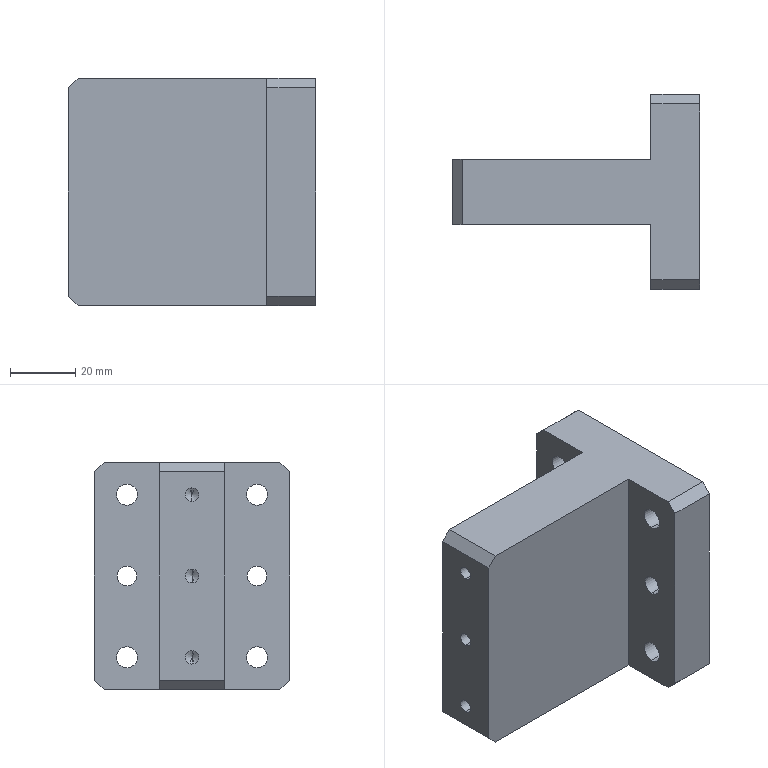Part | STEP file | 10-23 sliding mounting seat | 1 solid | 40 faces | box 76 x 60 x 70 mm | volume 144578 mm3 | cylinder 18 | plane 16 | cone 6 | commonest cylinder face diameters 6.5 x8 4.2 x6 6 x4
STEP:
#1=CARTESIAN_POINT('',(-48.6,0.,-27.1));
#2=VERTEX_POINT('',#1);
#3=CARTESIAN_POINT('',(-48.6,0.,-22.9));
#4=VERTEX_POINT('',#3);
#5=CARTESIAN_POINT('',(-48.6,0.,-25.));
#6=DIRECTION('',(-1.,0.,0.));
#7=DIRECTION('',(0.,0.,1.));
#8=AXIS2_PLACEMENT_3D('',#5,#6,#7);
#9=CIRCLE('',#8,2.1);
#10=EDGE_CURVE('',#2,#4,#9,.T.);
#11=ORIENTED_EDGE('',*,*,#10,.F.);
#12=CARTESIAN_POINT('',(-61.,0.,-27.1));
#13=VERTEX_POINT('',#12);
#14=CARTESIAN_POINT('',(-61.,0.,-27.1));
#15=DIRECTION('',(-1.,0.,0.));
#16=VECTOR('',#15,1000.);
#17=LINE('',#14,#16);
#18=EDGE_CURVE('',#2,#13,#17,.T.);
#19=ORIENTED_EDGE('',*,*,#18,.T.);
#20=CARTESIAN_POINT('',(-61.,0.,-22.9));
#21=VERTEX_POINT('',#20);
#22=CARTESIAN_POINT('',(-61.,0.,-25.));
#23=DIRECTION('',(-1.,0.,0.));
#24=DIRECTION('',(0.,0.,1.));
#25=AXIS2_PLACEMENT_3D('',#22,#23,#24);
#26=CIRCLE('',#25,2.1);
#27=EDGE_CURVE('',#13,#21,#26,.T.);
#28=ORIENTED_EDGE('',*,*,#27,.T.);
#29=CARTESIAN_POINT('',(-61.,0.,-22.9));
#30=DIRECTION('',(-1.,0.,0.));
#31=VECTOR('',#30,1000.);
#32=LINE('',#29,#31);
#33=EDGE_CURVE('',#4,#21,#32,.T.);
#34=ORIENTED_EDGE('',*,*,#33,.F.);
#35=EDGE_LOOP('',(#11,#19,#28,#34));
#36=FACE_OUTER_BOUND('',#35,.T.);
#37=CARTESIAN_POINT('',(-61.,0.,-25.));
#38=DIRECTION('',(-1.,0.,0.));
#39=DIRECTION('',(0.,0.,1.));
#40=AXIS2_PLACEMENT_3D('',#37,#38,#39);
#41=CYLINDRICAL_SURFACE('',#40,2.1);
#42=ADVANCED_FACE('',(#36),#41,.F.);
#43=CARTESIAN_POINT('',(-47.338,0.,-25.));
#44=VERTEX_POINT('',#43);
#45=CARTESIAN_POINT('',(-48.6,0.,-22.9));
#46=DIRECTION('',(-0.515,0.,0.8572));
#47=VECTOR('',#46,1000.);
#48=LINE('',#45,#47);
#49=EDGE_CURVE('',#44,#4,#48,.T.);
#50=ORIENTED_EDGE('',*,*,#49,.F.);
#51=CARTESIAN_POINT('',(-48.6,0.,-27.1));
#52=DIRECTION('',(-0.515,0.,-0.8572));
#53=VECTOR('',#52,1000.);
#54=LINE('',#51,#53);
#55=EDGE_CURVE('',#44,#2,#54,.T.);
#56=ORIENTED_EDGE('',*,*,#55,.T.);
#57=ORIENTED_EDGE('',*,*,#10,.T.);
#58=EDGE_LOOP('',(#50,#56,#57));
#59=FACE_OUTER_BOUND('',#58,.T.);
#60=CARTESIAN_POINT('',(-48.6,0.,-25.));
#61=DIRECTION('',(-1.,0.,0.));
#62=DIRECTION('',(0.,0.,1.));
#63=AXIS2_PLACEMENT_3D('',#60,#61,#62);
#64=CONICAL_SURFACE('',#63,2.1,1.03);
#65=ADVANCED_FACE('',(#59),#64,.F.);
#66=CARTESIAN_POINT('',(-48.6,0.,-2.1));
#67=VERTEX_POINT('',#66);
#68=CARTESIAN_POINT('',(-48.6,0.,2.1));
#69=VERTEX_POINT('',#68);
#70=CARTESIAN_POINT('',(-48.6,0.,0.));
#71=DIRECTION('',(-1.,0.,0.));
#72=DIRECTION('',(0.,0.,1.));
#73=AXIS2_PLACEMENT_3D('',#70,#71,#72);
#74=CIRCLE('',#73,2.1);
#75=EDGE_CURVE('',#67,#69,#74,.T.);
#76=ORIENTED_EDGE('',*,*,#75,.F.);
#77=CARTESIAN_POINT('',(-61.,0.,-2.1));
#78=VERTEX_POINT('',#77);
#79=CARTESIAN_POINT('',(-61.,0.,-2.1));
#80=DIRECTION('',(-1.,0.,0.));
#81=VECTOR('',#80,1000.);
#82=LINE('',#79,#81);
#83=EDGE_CURVE('',#67,#78,#82,.T.);
#84=ORIENTED_EDGE('',*,*,#83,.T.);
#85=CARTESIAN_POINT('',(-61.,0.,2.1));
#86=VERTEX_POINT('',#85);
#87=CARTESIAN_POINT('',(-61.,0.,0.));
#88=DIRECTION('',(-1.,0.,0.));
#89=DIRECTION('',(0.,0.,1.));
#90=AXIS2_PLACEMENT_3D('',#87,#88,#89);
#91=CIRCLE('',#90,2.1);
#92=EDGE_CURVE('',#78,#86,#91,.T.);
#93=ORIENTED_EDGE('',*,*,#92,.T.);
#94=CARTESIAN_POINT('',(-61.,0.,2.1));
#95=DIRECTION('',(-1.,0.,0.));
#96=VECTOR('',#95,1000.);
#97=LINE('',#94,#96);
#98=EDGE_CURVE('',#69,#86,#97,.T.);
#99=ORIENTED_EDGE('',*,*,#98,.F.);
#100=EDGE_LOOP('',(#76,#84,#93,#99));
#101=FACE_OUTER_BOUND('',#100,.T.);
#102=CARTESIAN_POINT('',(-61.,0.,0.));
#103=DIRECTION('',(-1.,0.,0.));
#104=DIRECTION('',(0.,0.,1.));
#105=AXIS2_PLACEMENT_3D('',#102,#103,#104);
#106=CYLINDRICAL_SURFACE('',#105,2.1);
#107=ADVANCED_FACE('',(#101),#106,.F.);
#108=CARTESIAN_POINT('',(-47.338,0.,0.));
#109=VERTEX_POINT('',#108);
#110=CARTESIAN_POINT('',(-48.6,0.,2.1));
#111=DIRECTION('',(-0.515,0.,0.8572));
#112=VECTOR('',#111,1000.);
#113=LINE('',#110,#112);
#114=EDGE_CURVE('',#109,#69,#113,.T.);
#115=ORIENTED_EDGE('',*,*,#114,.F.);
#116=CARTESIAN_POINT('',(-48.6,0.,-2.1));
#117=DIRECTION('',(-0.515,0.,-0.8572));
#118=VECTOR('',#117,1000.);
#119=LINE('',#116,#118);
#120=EDGE_CURVE('',#109,#67,#119,.T.);
#121=ORIENTED_EDGE('',*,*,#120,.T.);
#122=ORIENTED_EDGE('',*,*,#75,.T.);
#123=EDGE_LOOP('',(#115,#121,#122));
#124=FACE_OUTER_BOUND('',#123,.T.);
#125=CARTESIAN_POINT('',(-48.6,0.,0.));
#126=DIRECTION('',(-1.,0.,0.));
#127=DIRECTION('',(0.,0.,1.));
#128=AXIS2_PLACEMENT_3D('',#125,#126,#127);
#129=CONICAL_SURFACE('',#128,2.1,1.03);
#130=ADVANCED_FACE('',(#124),#129,.F.);
#131=CARTESIAN_POINT('',(-48.6,0.,22.9));
#132=VERTEX_POINT('',#131);
#133=CARTESIAN_POINT('',(-48.6,0.,27.1));
#134=VERTEX_POINT('',#133);
#135=CARTESIAN_POINT('',(-48.6,0.,25.));
#136=DIRECTION('',(-1.,0.,0.));
#137=DIRECTION('',(0.,0.,1.));
#138=AXIS2_PLACEMENT_3D('',#135,#136,#137);
#139=CIRCLE('',#138,2.1);
#140=EDGE_CURVE('',#132,#134,#139,.T.);
#141=ORIENTED_EDGE('',*,*,#140,.F.);
#142=CARTESIAN_POINT('',(-61.,0.,22.9));
#143=VERTEX_POINT('',#142);
#144=CARTESIAN_POINT('',(-61.,0.,22.9));
#145=DIRECTION('',(-1.,0.,0.));
#146=VECTOR('',#145,1000.);
#147=LINE('',#144,#146);
#148=EDGE_CURVE('',#132,#143,#147,.T.);
#149=ORIENTED_EDGE('',*,*,#148,.T.);
#150=CARTESIAN_POINT('',(-61.,0.,27.1));
#151=VERTEX_POINT('',#150);
#152=CARTESIAN_POINT('',(-61.,0.,25.));
#153=DIRECTION('',(-1.,0.,0.));
#154=DIRECTION('',(0.,0.,1.));
#155=AXIS2_PLACEMENT_3D('',#152,#153,#154);
#156=CIRCLE('',#155,2.1);
#157=EDGE_CURVE('',#143,#151,#156,.T.);
#158=ORIENTED_EDGE('',*,*,#157,.T.);
#159=CARTESIAN_POINT('',(-61.,0.,27.1));
#160=DIRECTION('',(-1.,0.,0.));
#161=VECTOR('',#160,1000.);
#162=LINE('',#159,#161);
#163=EDGE_CURVE('',#134,#151,#162,.T.);
#164=ORIENTED_EDGE('',*,*,#163,.F.);
#165=EDGE_LOOP('',(#141,#149,#158,#164));
#166=FACE_OUTER_BOUND('',#165,.T.);
#167=CARTESIAN_POINT('',(-61.,0.,25.));
#168=DIRECTION('',(-1.,0.,0.));
#169=DIRECTION('',(0.,0.,1.));
#170=AXIS2_PLACEMENT_3D('',#167,#168,#169);
#171=CYLINDRICAL_SURFACE('',#170,2.1);
#172=ADVANCED_FACE('',(#166),#171,.F.);
#173=CARTESIAN_POINT('',(-47.338,0.,25.));
#174=VERTEX_POINT('',#173);
#175=CARTESIAN_POINT('',(-48.6,0.,27.1));
#176=DIRECTION('',(-0.515,0.,0.8572));
#177=VECTOR('',#176,1000.);
#178=LINE('',#175,#177);
#179=EDGE_CURVE('',#174,#134,#178,.T.);
#180=ORIENTED_EDGE('',*,*,#179,.F.);
#181=CARTESIAN_POINT('',(-48.6,0.,22.9));
#182=DIRECTION('',(-0.515,0.,-0.8572));
#183=VECTOR('',#182,1000.);
#184=LINE('',#181,#183);
#185=EDGE_CURVE('',#174,#132,#184,.T.);
#186=ORIENTED_EDGE('',*,*,#185,.T.);
#187=ORIENTED_EDGE('',*,*,#140,.T.);
#188=EDGE_LOOP('',(#180,#186,#187));
#189=FACE_OUTER_BOUND('',#188,.T.);
#190=CARTESIAN_POINT('',(-48.6,0.,25.));
#191=DIRECTION('',(-1.,0.,0.));
#192=DIRECTION('',(0.,0.,1.));
#193=AXIS2_PLACEMENT_3D('',#190,#191,#192);
#194=CONICAL_SURFACE('',#193,2.1,1.03);
#195=ADVANCED_FACE('',(#189),#194,.F.);
#196=CARTESIAN_POINT('',(15.,20.,-3.));
#197=VERTEX_POINT('',#196);
#198=CARTESIAN_POINT('',(15.,20.,3.));
#199=VERTEX_POINT('',#198);
#200=CARTESIAN_POINT('',(15.,20.,0.));
#201=DIRECTION('',(-1.,0.,0.));
#202=DIRECTION('',(0.,0.,1.));
#203=AXIS2_PLACEMENT_3D('',#200,#201,#202);
#204=CIRCLE('',#203,3.);
#205=EDGE_CURVE('',#197,#199,#204,.T.);
#206=ORIENTED_EDGE('',*,*,#205,.F.);
#207=CARTESIAN_POINT('',(0.,20.,-3.));
#208=VERTEX_POINT('',#207);
#209=CARTESIAN_POINT('',(0.,20.,-3.));
#210=DIRECTION('',(-1.,0.,0.));
#211=VECTOR('',#210,1000.);
#212=LINE('',#209,#211);
#213=EDGE_CURVE('',#197,#208,#212,.T.);
#214=ORIENTED_EDGE('',*,*,#213,.T.);
#215=CARTESIAN_POINT('',(0.,20.,3.));
#216=VERTEX_POINT('',#215);
#217=CARTESIAN_POINT('',(0.,20.,0.));
#218=DIRECTION('',(-1.,0.,0.));
#219=DIRECTION('',(0.,0.,1.));
#220=AXIS2_PLACEMENT_3D('',#217,#218,#219);
#221=CIRCLE('',#220,3.);
#222=EDGE_CURVE('',#208,#216,#221,.T.);
#223=ORIENTED_EDGE('',*,*,#222,.T.);
#224=CARTESIAN_POINT('',(0.,20.,3.));
#225=DIRECTION('',(-1.,0.,0.));
#226=VECTOR('',#225,1000.);
#227=LINE('',#224,#226);
#228=EDGE_CURVE('',#199,#216,#227,.T.);
#229=ORIENTED_EDGE('',*,*,#228,.F.);
#230=EDGE_LOOP('',(#206,#214,#223,#229));
#231=FACE_OUTER_BOUND('',#230,.T.);
#232=CARTESIAN_POINT('',(0.,20.,0.));
#233=DIRECTION('',(-1.,0.,0.));
#234=DIRECTION('',(0.,0.,1.));
#235=AXIS2_PLACEMENT_3D('',#232,#233,#234);
#236=CYLINDRICAL_SURFACE('',#235,3.);
#237=ADVANCED_FACE('',(#231),#236,.F.);
#238=CARTESIAN_POINT('',(15.,-20.,-3.));
#239=VERTEX_POINT('',#238);
#240=CARTESIAN_POINT('',(15.,-20.,3.));
#241=VERTEX_POINT('',#240);
#242=CARTESIAN_POINT('',(15.,-20.,0.));
#243=DIRECTION('',(-1.,0.,0.));
#244=DIRECTION('',(0.,0.,1.));
#245=AXIS2_PLACEMENT_3D('',#242,#243,#244);
#246=CIRCLE('',#245,3.);
#247=EDGE_CURVE('',#239,#241,#246,.T.);
#248=ORIENTED_EDGE('',*,*,#247,.F.);
#249=CARTESIAN_POINT('',(0.,-20.,-3.));
#250=VERTEX_POINT('',#249);
#251=CARTESIAN_POINT('',(0.,-20.,-3.));
#252=DIRECTION('',(-1.,0.,0.));
#253=VECTOR('',#252,1000.);
#254=LINE('',#251,#253);
#255=EDGE_CURVE('',#239,#250,#254,.T.);
#256=ORIENTED_EDGE('',*,*,#255,.T.);
#257=CARTESIAN_POINT('',(0.,-20.,3.));
#258=VERTEX_POINT('',#257);
#259=CARTESIAN_POINT('',(0.,-20.,0.));
#260=DIRECTION('',(-1.,0.,0.));
#261=DIRECTION('',(0.,0.,1.));
#262=AXIS2_PLACEMENT_3D('',#259,#260,#261);
#263=CIRCLE('',#262,3.);
#264=EDGE_CURVE('',#250,#258,#263,.T.);
#265=ORIENTED_EDGE('',*,*,#264,.T.);
#266=CARTESIAN_POINT('',(0.,-20.,3.));
#267=DIRECTION('',(-1.,0.,0.));
#268=VECTOR('',#267,1000.);
#269=LINE('',#266,#268);
#270=EDGE_CURVE('',#241,#258,#269,.T.);
#271=ORIENTED_EDGE('',*,*,#270,.F.);
#272=EDGE_LOOP('',(#248,#256,#265,#271));
#273=FACE_OUTER_BOUND('',#272,.T.);
#274=CARTESIAN_POINT('',(0.,-20.,0.));
#275=DIRECTION('',(-1.,0.,0.));
#276=DIRECTION('',(0.,0.,1.));
#277=AXIS2_PLACEMENT_3D('',#274,#275,#276);
#278=CYLINDRICAL_SURFACE('',#277,3.);
#279=ADVANCED_FACE('',(#273),#278,.F.);
#280=CARTESIAN_POINT('',(15.,20.,-28.25));
#281=VERTEX_POINT('',#280);
#282=CARTESIAN_POINT('',(15.,20.,-21.75));
#283=VERTEX_POINT('',#282);
#284=CARTESIAN_POINT('',(15.,20.,-25.));
#285=DIRECTION('',(-1.,0.,0.));
#286=DIRECTION('',(0.,0.,1.));
#287=AXIS2_PLACEMENT_3D('',#284,#285,#286);
#288=CIRCLE('',#287,3.25);
#289=EDGE_CURVE('',#281,#283,#288,.T.);
#290=ORIENTED_EDGE('',*,*,#289,.F.);
#291=CARTESIAN_POINT('',(0.,20.,-28.25));
#292=VERTEX_POINT('',#291);
#293=CARTESIAN_POINT('',(0.,20.,-28.25));
#294=DIRECTION('',(-1.,0.,0.));
#295=VECTOR('',#294,1000.);
#296=LINE('',#293,#295);
#297=EDGE_CURVE('',#281,#292,#296,.T.);
#298=ORIENTED_EDGE('',*,*,#297,.T.);
#299=CARTESIAN_POINT('',(0.,20.,-21.75));
#300=VERTEX_POINT('',#299);
#301=CARTESIAN_POINT('',(0.,20.,-25.));
#302=DIRECTION('',(-1.,0.,0.));
#303=DIRECTION('',(0.,0.,1.));
#304=AXIS2_PLACEMENT_3D('',#301,#302,#303);
#305=CIRCLE('',#304,3.25);
#306=EDGE_CURVE('',#292,#300,#305,.T.);
#307=ORIENTED_EDGE('',*,*,#306,.T.);
#308=CARTESIAN_POINT('',(0.,20.,-21.75));
#309=DIRECTION('',(-1.,0.,0.));
#310=VECTOR('',#309,1000.);
#311=LINE('',#308,#310);
#312=EDGE_CURVE('',#283,#300,#311,.T.);
#313=ORIENTED_EDGE('',*,*,#312,.F.);
#314=EDGE_LOOP('',(#290,#298,#307,#313));
#315=FACE_OUTER_BOUND('',#314,.T.);
#316=CARTESIAN_POINT('',(0.,20.,-25.));
#317=DIRECTION('',(-1.,0.,0.));
#318=DIRECTION('',(0.,0.,1.));
#319=AXIS2_PLACEMENT_3D('',#316,#317,#318);
#320=CYLINDRICAL_SURFACE('',#319,3.25);
#321=ADVANCED_FACE('',(#315),#320,.F.);
#322=CARTESIAN_POINT('',(15.,20.,21.75));
#323=VERTEX_POINT('',#322);
#324=CARTESIAN_POINT('',(15.,20.,28.25));
#325=VERTEX_POINT('',#324);
#326=CARTESIAN_POINT('',(15.,20.,25.));
#327=DIRECTION('',(-1.,0.,0.));
#328=DIRECTION('',(0.,0.,1.));
#329=AXIS2_PLACEMENT_3D('',#326,#327,#328);
#330=CIRCLE('',#329,3.25);
#331=EDGE_CURVE('',#323,#325,#330,.T.);
#332=ORIENTED_EDGE('',*,*,#331,.F.);
#333=CARTESIAN_POINT('',(0.,20.,21.75));
#334=VERTEX_POINT('',#333);
#335=CARTESIAN_POINT('',(0.,20.,21.75));
#336=DIRECTION('',(-1.,0.,0.));
#337=VECTOR('',#336,1000.);
#338=LINE('',#335,#337);
#339=EDGE_CURVE('',#323,#334,#338,.T.);
#340=ORIENTED_EDGE('',*,*,#339,.T.);
#341=CARTESIAN_POINT('',(0.,20.,28.25));
#342=VERTEX_POINT('',#341);
#343=CARTESIAN_POINT('',(0.,20.,25.));
#344=DIRECTION('',(-1.,0.,0.));
#345=DIRECTION('',(0.,0.,1.));
#346=AXIS2_PLACEMENT_3D('',#343,#344,#345);
#347=CIRCLE('',#346,3.25);
#348=EDGE_CURVE('',#334,#342,#347,.T.);
#349=ORIENTED_EDGE('',*,*,#348,.T.);
#350=CARTESIAN_POINT('',(0.,20.,28.25));
#351=DIRECTION('',(-1.,0.,0.));
#352=VECTOR('',#351,1000.);
#353=LINE('',#350,#352);
#354=EDGE_CURVE('',#325,#342,#353,.T.);
#355=ORIENTED_EDGE('',*,*,#354,.F.);
#356=EDGE_LOOP('',(#332,#340,#349,#355));
#357=FACE_OUTER_BOUND('',#356,.T.);
#358=CARTESIAN_POINT('',(0.,20.,25.));
#359=DIRECTION('',(-1.,0.,0.));
#360=DIRECTION('',(0.,0.,1.));
#361=AXIS2_PLACEMENT_3D('',#358,#359,#360);
#362=CYLINDRICAL_SURFACE('',#361,3.25);
#363=ADVANCED_FACE('',(#357),#362,.F.);
#364=CARTESIAN_POINT('',(15.,-20.,-28.25));
#365=VERTEX_POINT('',#364);
#366=CARTESIAN_POINT('',(15.,-20.,-21.75));
#367=VERTEX_POINT('',#366);
#368=CARTESIAN_POINT('',(15.,-20.,-25.));
#369=DIRECTION('',(-1.,0.,0.));
#370=DIRECTION('',(0.,0.,1.));
#371=AXIS2_PLACEMENT_3D('',#368,#369,#370);
#372=CIRCLE('',#371,3.25);
#373=EDGE_CURVE('',#365,#367,#372,.T.);
#374=ORIENTED_EDGE('',*,*,#373,.F.);
#375=CARTESIAN_POINT('',(0.,-20.,-28.25));
#376=VERTEX_POINT('',#375);
#377=CARTESIAN_POINT('',(0.,-20.,-28.25));
#378=DIRECTION('',(-1.,0.,0.));
#379=VECTOR('',#378,1000.);
#380=LINE('',#377,#379);
#381=EDGE_CURVE('',#365,#376,#380,.T.);
#382=ORIENTED_EDGE('',*,*,#381,.T.);
#383=CARTESIAN_POINT('',(0.,-20.,-21.75));
#384=VERTEX_POINT('',#383);
#385=CARTESIAN_POINT('',(0.,-20.,-25.));
#386=DIRECTION('',(-1.,0.,0.));
#387=DIRECTION('',(0.,0.,1.));
#388=AXIS2_PLACEMENT_3D('',#385,#386,#387);
#389=CIRCLE('',#388,3.25);
#390=EDGE_CURVE('',#376,#384,#389,.T.);
#391=ORIENTED_EDGE('',*,*,#390,.T.);
#392=CARTESIAN_POINT('',(0.,-20.,-21.75));
#393=DIRECTION('',(-1.,0.,0.));
#394=VECTOR('',#393,1000.);
#395=LINE('',#392,#394);
#396=EDGE_CURVE('',#367,#384,#395,.T.);
#397=ORIENTED_EDGE('',*,*,#396,.F.);
#398=EDGE_LOOP('',(#374,#382,#391,#397));
#399=FACE_OUTER_BOUND('',#398,.T.);
#400=CARTESIAN_POINT('',(0.,-20.,-25.));
#401=DIRECTION('',(-1.,0.,0.));
#402=DIRECTION('',(0.,0.,1.));
#403=AXIS2_PLACEMENT_3D('',#400,#401,#402);
#404=CYLINDRICAL_SURFACE('',#403,3.25);
#405=ADVANCED_FACE('',(#399),#404,.F.);
#406=CARTESIAN_POINT('',(15.,-20.,21.75));
#407=VERTEX_POINT('',#406);
#408=CARTESIAN_POINT('',(15.,-20.,28.25));
#409=VERTEX_POINT('',#408);
#410=CARTESIAN_POINT('',(15.,-20.,25.));
#411=DIRECTION('',(-1.,0.,0.));
#412=DIRECTION('',(0.,0.,1.));
#413=AXIS2_PLACEMENT_3D('',#410,#411,#412);
#414=CIRCLE('',#413,3.25);
#415=EDGE_CURVE('',#407,#409,#414,.T.);
#416=ORIENTED_EDGE('',*,*,#415,.F.);
#417=CARTESIAN_POINT('',(0.,-20.,21.75));
#418=VERTEX_POINT('',#417);
#419=CARTESIAN_POINT('',(0.,-20.,21.75));
#420=DIRECTION('',(-1.,0.,0.));
#421=VECTOR('',#420,1000.);
#422=LINE('',#419,#421);
#423=EDGE_CURVE('',#407,#418,#422,.T.);
#424=ORIENTED_EDGE('',*,*,#423,.T.);
#425=CARTESIAN_POINT('',(0.,-20.,28.25));
#426=VERTEX_POINT('',#425);
#427=CARTESIAN_POINT('',(0.,-20.,25.));
#428=DIRECTION('',(-1.,0.,0.));
#429=DIRECTION('',(0.,0.,1.));
#430=AXIS2_PLACEMENT_3D('',#427,#428,#429);
#431=CIRCLE('',#430,3.25);
#432=EDGE_CURVE('',#418,#426,#431,.T.);
#433=ORIENTED_EDGE('',*,*,#432,.T.);
#434=CARTESIAN_POINT('',(0.,-20.,28.25));
#435=DIRECTION('',(-1.,0.,0.));
#436=VECTOR('',#435,1000.);
#437=LINE('',#434,#436);
#438=EDGE_CURVE('',#409,#426,#437,.T.);
#439=ORIENTED_EDGE('',*,*,#438,.F.);
#440=EDGE_LOOP('',(#416,#424,#433,#439));
#441=FACE_OUTER_BOUND('',#440,.T.);
#442=CARTESIAN_POINT('',(0.,-20.,25.));
#443=DIRECTION('',(-1.,0.,0.));
#444=DIRECTION('',(0.,0.,1.));
#445=AXIS2_PLACEMENT_3D('',#442,#443,#444);
#446=CYLINDRICAL_SURFACE('',#445,3.25);
#447=ADVANCED_FACE('',(#441),#446,.F.);
#448=CARTESIAN_POINT('',(0.,20.,0.));
#449=DIRECTION('',(-1.,0.,0.));
#450=DIRECTION('',(0.,0.,1.));
#451=AXIS2_PLACEMENT_3D('',#448,#449,#450);
#452=CIRCLE('',#451,3.);
#453=EDGE_CURVE('',#216,#208,#452,.T.);
#454=ORIENTED_EDGE('',*,*,#453,.F.);
#455=ORIENTED_EDGE('',*,*,#222,.F.);
#456=EDGE_LOOP('',(#454,#455));
#457=FACE_BOUND('',#456,.T.);
#458=CARTESIAN_POINT('',(0.,20.,-25.));
#459=DIRECTION('',(-1.,0.,0.));
#460=DIRECTION('',(0.,0.,1.));
#461=AXIS2_PLACEMENT_3D('',#458,#459,#460);
#462=CIRCLE('',#461,3.25);
#463=EDGE_CURVE('',#300,#292,#462,.T.);
#464=ORIENTED_EDGE('',*,*,#463,.F.);
#465=ORIENTED_EDGE('',*,*,#306,.F.);
#466=EDGE_LOOP('',(#464,#465));
#467=FACE_BOUND('',#466,.T.);
#468=CARTESIAN_POINT('',(0.,20.,25.));
#469=DIRECTION('',(-1.,0.,0.));
#470=DIRECTION('',(0.,0.,1.));
#471=AXIS2_PLACEMENT_3D('',#468,#469,#470);
#472=CIRCLE('',#471,3.25);
#473=EDGE_CURVE('',#342,#334,#472,.T.);
#474=ORIENTED_EDGE('',*,*,#473,.F.);
#475=ORIENTED_EDGE('',*,*,#348,.F.);
#476=EDGE_LOOP('',(#474,#475));
#477=FACE_BOUND('',#476,.T.);
#478=CARTESIAN_POINT('',(0.,30.,32.));
#479=VERTEX_POINT('',#478);
#480=CARTESIAN_POINT('',(0.,30.,-32.));
#481=VERTEX_POINT('',#480);
#482=CARTESIAN_POINT('',(0.,30.,35.));
#483=DIRECTION('',(0.,0.,-1.));
#484=VECTOR('',#483,1000.);
#485=LINE('',#482,#484);
#486=EDGE_CURVE('',#479,#481,#485,.T.);
#487=ORIENTED_EDGE('',*,*,#486,.T.);
#488=CARTESIAN_POINT('',(0.,27.,-35.));
#489=VERTEX_POINT('',#488);
#490=CARTESIAN_POINT('',(0.,30.,-32.));
#491=DIRECTION('',(0.,-0.7071,-0.7071));
#492=VECTOR('',#491,1000.);
#493=LINE('',#490,#492);
#494=EDGE_CURVE('',#481,#489,#493,.T.);
#495=ORIENTED_EDGE('',*,*,#494,.T.);
#496=CARTESIAN_POINT('',(0.,10.,-35.));
#497=VERTEX_POINT('',#496);
#498=CARTESIAN_POINT('',(0.,10.,-35.));
#499=DIRECTION('',(0.,-1.,0.));
#500=VECTOR('',#499,1000.);
#501=LINE('',#498,#500);
#502=EDGE_CURVE('',#489,#497,#501,.T.);
#503=ORIENTED_EDGE('',*,*,#502,.T.);
#504=CARTESIAN_POINT('',(0.,10.,35.));
#505=VERTEX_POINT('',#504);
#506=CARTESIAN_POINT('',(0.,10.,35.));
#507=DIRECTION('',(0.,0.,-1.));
#508=VECTOR('',#507,1000.);
#509=LINE('',#506,#508);
#510=EDGE_CURVE('',#505,#497,#509,.T.);
#511=ORIENTED_EDGE('',*,*,#510,.F.);
#512=CARTESIAN_POINT('',(0.,27.,35.));
#513=VERTEX_POINT('',#512);
#514=CARTESIAN_POINT('',(0.,10.,35.));
#515=DIRECTION('',(0.,-1.,0.));
#516=VECTOR('',#515,1000.);
#517=LINE('',#514,#516);
#518=EDGE_CURVE('',#513,#505,#517,.T.);
#519=ORIENTED_EDGE('',*,*,#518,.F.);
#520=CARTESIAN_POINT('',(0.,27.,35.));
#521=DIRECTION('',(0.,0.7071,-0.7071));
#522=VECTOR('',#521,1000.);
#523=LINE('',#520,#522);
#524=EDGE_CURVE('',#513,#479,#523,.T.);
#525=ORIENTED_EDGE('',*,*,#524,.T.);
#526=EDGE_LOOP('',(#487,#495,#503,#511,#519,#525));
#527=FACE_OUTER_BOUND('',#526,.T.);
#528=CARTESIAN_POINT('',(0.,10.,35.));
#529=DIRECTION('',(1.,0.,0.));
#530=DIRECTION('',(0.,0.,-1.));
#531=AXIS2_PLACEMENT_3D('',#528,#529,#530);
#532=PLANE('',#531);
#533=ADVANCED_FACE('',(#457,#467,#477,#527),#532,.F.);
#534=CARTESIAN_POINT('',(-58.,10.,-35.));
#535=VERTEX_POINT('',#534);
#536=CARTESIAN_POINT('',(-61.,10.,-35.));
#537=DIRECTION('',(-1.,0.,0.));
#538=VECTOR('',#537,1000.);
#539=LINE('',#536,#538);
#540=EDGE_CURVE('',#497,#535,#539,.T.);
#541=ORIENTED_EDGE('',*,*,#540,.T.);
#542=CARTESIAN_POINT('',(-61.,10.,-32.));
#543=VERTEX_POINT('',#542);
#544=CARTESIAN_POINT('',(-61.,10.,-32.));
#545=DIRECTION('',(-0.7071,0.,0.7071));
#546=VECTOR('',#545,1000.);
#547=LINE('',#544,#546);
#548=EDGE_CURVE('',#535,#543,#547,.T.);
#549=ORIENTED_EDGE('',*,*,#548,.T.);
#550=CARTESIAN_POINT('',(-61.,10.,32.));
#551=VERTEX_POINT('',#550);
#552=CARTESIAN_POINT('',(-61.,10.,35.));
#553=DIRECTION('',(0.,0.,-1.));
#554=VECTOR('',#553,1000.);
#555=LINE('',#552,#554);
#556=EDGE_CURVE('',#551,#543,#555,.T.);
#557=ORIENTED_EDGE('',*,*,#556,.F.);
#558=CARTESIAN_POINT('',(-58.,10.,35.));
#559=VERTEX_POINT('',#558);
#560=CARTESIAN_POINT('',(-58.,10.,35.));
#561=DIRECTION('',(0.7071,0.,0.7071));
#562=VECTOR('',#561,1000.);
#563=LINE('',#560,#562);
#564=EDGE_CURVE('',#551,#559,#563,.T.);
#565=ORIENTED_EDGE('',*,*,#564,.T.);
#566=CARTESIAN_POINT('',(-61.,10.,35.));
#567=DIRECTION('',(-1.,0.,0.));
#568=VECTOR('',#567,1000.);
#569=LINE('',#566,#568);
#570=EDGE_CURVE('',#505,#559,#569,.T.);
#571=ORIENTED_EDGE('',*,*,#570,.F.);
#572=ORIENTED_EDGE('',*,*,#510,.T.);
#573=EDGE_LOOP('',(#541,#549,#557,#565,#571,#572));
#574=FACE_OUTER_BOUND('',#573,.T.);
#575=CARTESIAN_POINT('',(-61.,10.,35.));
#576=DIRECTION('',(0.,-1.,0.));
#577=DIRECTION('',(0.,0.,-1.));
#578=AXIS2_PLACEMENT_3D('',#575,#576,#577);
#579=PLANE('',#578);
#580=ADVANCED_FACE('',(#574),#579,.F.);
#581=CARTESIAN_POINT('',(-61.,0.,-25.));
#582=DIRECTION('',(-1.,0.,0.));
#583=DIRECTION('',(0.,0.,1.));
#584=AXIS2_PLACEMENT_3D('',#581,#582,#583);
#585=CIRCLE('',#584,2.1);
#586=EDGE_CURVE('',#21,#13,#585,.T.);
#587=ORIENTED_EDGE('',*,*,#586,.F.);
#588=ORIENTED_EDGE('',*,*,#27,.F.);
#589=EDGE_LOOP('',(#587,#588));
#590=FACE_BOUND('',#589,.T.);
#591=CARTESIAN_POINT('',(-61.,0.,0.));
#592=DIRECTION('',(-1.,0.,0.));
#593=DIRECTION('',(0.,0.,1.));
#594=AXIS2_PLACEMENT_3D('',#591,#592,#593);
#595=CIRCLE('',#594,2.1);
#596=EDGE_CURVE('',#86,#78,#595,.T.);
#597=ORIENTED_EDGE('',*,*,#596,.F.);
#598=ORIENTED_EDGE('',*,*,#92,.F.);
#599=EDGE_LOOP('',(#597,#598));
#600=FACE_BOUND('',#599,.T.);
#601=CARTESIAN_POINT('',(-61.,0.,25.));
#602=DIRECTION('',(-1.,0.,0.));
#603=DIRECTION('',(0.,0.,1.));
#604=AXIS2_PLACEMENT_3D('',#601,#602,#603);
#605=CIRCLE('',#604,2.1);
#606=EDGE_CURVE('',#151,#143,#605,.T.);
#607=ORIENTED_EDGE('',*,*,#606,.F.);
#608=ORIENTED_EDGE('',*,*,#157,.F.);
#609=EDGE_LOOP('',(#607,#608));
#610=FACE_BOUND('',#609,.T.);
#611=ORIENTED_EDGE('',*,*,#556,.T.);
#612=CARTESIAN_POINT('',(-61.,-10.,-32.));
#613=VERTEX_POINT('',#612);
#614=CARTESIAN_POINT('',(-61.,-10.,-32.));
#615=DIRECTION('',(0.,-1.,0.));
#616=VECTOR('',#615,1000.);
#617=LINE('',#614,#616);
#618=EDGE_CURVE('',#543,#613,#617,.T.);
#619=ORIENTED_EDGE('',*,*,#618,.T.);
#620=CARTESIAN_POINT('',(-61.,-10.,32.));
#621=VERTEX_POINT('',#620);
#622=CARTESIAN_POINT('',(-61.,-10.,35.));
#623=DIRECTION('',(0.,0.,-1.));
#624=VECTOR('',#623,1000.);
#625=LINE('',#622,#624);
#626=EDGE_CURVE('',#621,#613,#625,.T.);
#627=ORIENTED_EDGE('',*,*,#626,.F.);
#628=CARTESIAN_POINT('',(-61.,-10.,32.));
#629=DIRECTION('',(0.,1.,0.));
#630=VECTOR('',#629,1000.);
#631=LINE('',#628,#630);
#632=EDGE_CURVE('',#621,#551,#631,.T.);
#633=ORIENTED_EDGE('',*,*,#632,.T.);
#634=EDGE_LOOP('',(#611,#619,#627,#633));
#635=FACE_OUTER_BOUND('',#634,.T.);
#636=CARTESIAN_POINT('',(-61.,-10.,35.));
#637=DIRECTION('',(1.,0.,0.));
#638=DIRECTION('',(0.,0.,-1.));
#639=AXIS2_PLACEMENT_3D('',#636,#637,#638);
#640=PLANE('',#639);
#641=ADVANCED_FACE('',(#590,#600,#610,#635),#640,.F.);
#642=ORIENTED_EDGE('',*,*,#626,.T.);
#643=CARTESIAN_POINT('',(-58.,-10.,-35.));
#644=VERTEX_POINT('',#643);
#645=CARTESIAN_POINT('',(-61.,-10.,-32.));
#646=DIRECTION('',(0.7071,0.,-0.7071));
#647=VECTOR('',#646,1000.);
#648=LINE('',#645,#647);
#649=EDGE_CURVE('',#613,#644,#648,.T.);
#650=ORIENTED_EDGE('',*,*,#649,.T.);
#651=CARTESIAN_POINT('',(0.,-10.,-35.));
#652=VERTEX_POINT('',#651);
#653=CARTESIAN_POINT('',(0.,-10.,-35.));
#654=DIRECTION('',(1.,0.,0.));
#655=VECTOR('',#654,1000.);
#656=LINE('',#653,#655);
#657=EDGE_CURVE('',#644,#652,#656,.T.);
#658=ORIENTED_EDGE('',*,*,#657,.T.);
#659=CARTESIAN_POINT('',(0.,-10.,35.));
#660=VERTEX_POINT('',#659);
#661=CARTESIAN_POINT('',(0.,-10.,35.));
#662=DIRECTION('',(0.,0.,-1.));
#663=VECTOR('',#662,1000.);
#664=LINE('',#661,#663);
#665=EDGE_CURVE('',#660,#652,#664,.T.);
#666=ORIENTED_EDGE('',*,*,#665,.F.);
#667=CARTESIAN_POINT('',(-58.,-10.,35.));
#668=VERTEX_POINT('',#667);
#669=CARTESIAN_POINT('',(0.,-10.,35.));
#670=DIRECTION('',(1.,0.,0.));
#671=VECTOR('',#670,1000.);
#672=LINE('',#669,#671);
#673=EDGE_CURVE('',#668,#660,#672,.T.);
#674=ORIENTED_EDGE('',*,*,#673,.F.);
#675=CARTESIAN_POINT('',(-58.,-10.,35.));
#676=DIRECTION('',(-0.7071,0.,-0.7071));
#677=VECTOR('',#676,1000.);
#678=LINE('',#675,#677);
#679=EDGE_CURVE('',#668,#621,#678,.T.);
#680=ORIENTED_EDGE('',*,*,#679,.T.);
#681=EDGE_LOOP('',(#642,#650,#658,#666,#674,#680));
#682=FACE_OUTER_BOUND('',#681,.T.);
#683=CARTESIAN_POINT('',(0.,-10.,35.));
#684=DIRECTION('',(0.,1.,0.));
#685=DIRECTION('',(0.,0.,1.));
#686=AXIS2_PLACEMENT_3D('',#683,#684,#685);
#687=PLANE('',#686);
#688=ADVANCED_FACE('',(#682),#687,.F.);
#689=CARTESIAN_POINT('',(0.,-20.,0.));
#690=DIRECTION('',(-1.,0.,0.));
#691=DIRECTION('',(0.,0.,1.));
#692=AXIS2_PLACEMENT_3D('',#689,#690,#691);
#693=CIRCLE('',#692,3.);
#694=EDGE_CURVE('',#258,#250,#693,.T.);
#695=ORIENTED_EDGE('',*,*,#694,.F.);
#696=ORIENTED_EDGE('',*,*,#264,.F.);
#697=EDGE_LOOP('',(#695,#696));
#698=FACE_BOUND('',#697,.T.);
#699=CARTESIAN_POINT('',(0.,-20.,-25.));
#700=DIRECTION('',(-1.,0.,0.));
#701=DIRECTION('',(0.,0.,1.));
#702=AXIS2_PLACEMENT_3D('',#699,#700,#701);
#703=CIRCLE('',#702,3.25);
#704=EDGE_CURVE('',#384,#376,#703,.T.);
#705=ORIENTED_EDGE('',*,*,#704,.F.);
#706=ORIENTED_EDGE('',*,*,#390,.F.);
#707=EDGE_LOOP('',(#705,#706));
#708=FACE_BOUND('',#707,.T.);
#709=CARTESIAN_POINT('',(0.,-20.,25.));
#710=DIRECTION('',(-1.,0.,0.));
#711=DIRECTION('',(0.,0.,1.));
#712=AXIS2_PLACEMENT_3D('',#709,#710,#711);
#713=CIRCLE('',#712,3.25);
#714=EDGE_CURVE('',#426,#418,#713,.T.);
#715=ORIENTED_EDGE('',*,*,#714,.F.);
#716=ORIENTED_EDGE('',*,*,#432,.F.);
#717=EDGE_LOOP('',(#715,#716));
#718=FACE_BOUND('',#717,.T.);
#719=CARTESIAN_POINT('',(0.,-30.,32.));
#720=VERTEX_POINT('',#719);
#721=CARTESIAN_POINT('',(0.,-30.,-32.));
#722=VERTEX_POINT('',#721);
#723=CARTESIAN_POINT('',(0.,-30.,35.));
#724=DIRECTION('',(0.,0.,-1.));
#725=VECTOR('',#724,1000.);
#726=LINE('',#723,#725);
#727=EDGE_CURVE('',#720,#722,#726,.T.);
#728=ORIENTED_EDGE('',*,*,#727,.F.);
#729=CARTESIAN_POINT('',(0.,-27.,35.));
#730=VERTEX_POINT('',#729);
#731=CARTESIAN_POINT('',(0.,-27.,35.));
#732=DIRECTION('',(0.,0.7071,0.7071));
#733=VECTOR('',#732,1000.);
#734=LINE('',#731,#733);
#735=EDGE_CURVE('',#720,#730,#734,.T.);
#736=ORIENTED_EDGE('',*,*,#735,.T.);
#737=CARTESIAN_POINT('',(0.,-30.,35.));
#738=DIRECTION('',(0.,-1.,0.));
#739=VECTOR('',#738,1000.);
#740=LINE('',#737,#739);
#741=EDGE_CURVE('',#660,#730,#740,.T.);
#742=ORIENTED_EDGE('',*,*,#741,.F.);
#743=ORIENTED_EDGE('',*,*,#665,.T.);
#744=CARTESIAN_POINT('',(0.,-27.,-35.));
#745=VERTEX_POINT('',#744);
#746=CARTESIAN_POINT('',(0.,-30.,-35.));
#747=DIRECTION('',(0.,-1.,0.));
#748=VECTOR('',#747,1000.);
#749=LINE('',#746,#748);
#750=EDGE_CURVE('',#652,#745,#749,.T.);
#751=ORIENTED_EDGE('',*,*,#750,.T.);
#752=CARTESIAN_POINT('',(0.,-30.,-32.));
#753=DIRECTION('',(0.,-0.7071,0.7071));
#754=VECTOR('',#753,1000.);
#755=LINE('',#752,#754);
#756=EDGE_CURVE('',#745,#722,#755,.T.);
#757=ORIENTED_EDGE('',*,*,#756,.T.);
#758=EDGE_LOOP('',(#728,#736,#742,#743,#751,#757));
#759=FACE_OUTER_BOUND('',#758,.T.);
#760=CARTESIAN_POINT('',(0.,-30.,35.));
#761=DIRECTION('',(1.,0.,0.));
#762=DIRECTION('',(0.,0.,-1.));
#763=AXIS2_PLACEMENT_3D('',#760,#761,#762);
#764=PLANE('',#763);
#765=ADVANCED_FACE('',(#698,#708,#718,#759),#764,.F.);
#766=CARTESIAN_POINT('',(15.,-30.,32.));
#767=VERTEX_POINT('',#766);
#768=CARTESIAN_POINT('',(15.,-30.,-32.));
#769=VERTEX_POINT('',#768);
#770=CARTESIAN_POINT('',(15.,-30.,35.));
#771=DIRECTION('',(0.,0.,-1.));
#772=VECTOR('',#771,1000.);
#773=LINE('',#770,#772);
#774=EDGE_CURVE('',#767,#769,#773,.T.);
#775=ORIENTED_EDGE('',*,*,#774,.F.);
#776=CARTESIAN_POINT('',(15.,-30.,32.));
#777=DIRECTION('',(-1.,0.,0.));
#778=VECTOR('',#777,1000.);
#779=LINE('',#776,#778);
#780=EDGE_CURVE('',#767,#720,#779,.T.);
#781=ORIENTED_EDGE('',*,*,#780,.T.);
#782=ORIENTED_EDGE('',*,*,#727,.T.);
#783=CARTESIAN_POINT('',(15.,-30.,-32.));
#784=DIRECTION('',(1.,0.,0.));
#785=VECTOR('',#784,1000.);
#786=LINE('',#783,#785);
#787=EDGE_CURVE('',#722,#769,#786,.T.);
#788=ORIENTED_EDGE('',*,*,#787,.T.);
#789=EDGE_LOOP('',(#775,#781,#782,#788));
#790=FACE_OUTER_BOUND('',#789,.T.);
#791=CARTESIAN_POINT('',(15.,-30.,35.));
#792=DIRECTION('',(0.,1.,0.));
#793=DIRECTION('',(-1.,0.,0.));
#794=AXIS2_PLACEMENT_3D('',#791,#792,#793);
#795=PLANE('',#794);
#796=ADVANCED_FACE('',(#790),#795,.F.);
#797=CARTESIAN_POINT('',(15.,20.,0.));
#798=DIRECTION('',(-1.,0.,0.));
#799=DIRECTION('',(0.,0.,1.));
#800=AXIS2_PLACEMENT_3D('',#797,#798,#799);
#801=CIRCLE('',#800,3.);
#802=EDGE_CURVE('',#199,#197,#801,.T.);
#803=ORIENTED_EDGE('',*,*,#802,.T.);
#804=ORIENTED_EDGE('',*,*,#205,.T.);
#805=EDGE_LOOP('',(#803,#804));
#806=FACE_BOUND('',#805,.T.);
#807=CARTESIAN_POINT('',(15.,-20.,0.));
#808=DIRECTION('',(-1.,0.,0.));
#809=DIRECTION('',(0.,0.,1.));
#810=AXIS2_PLACEMENT_3D('',#807,#808,#809);
#811=CIRCLE('',#810,3.);
#812=EDGE_CURVE('',#241,#239,#811,.T.);
#813=ORIENTED_EDGE('',*,*,#812,.T.);
#814=ORIENTED_EDGE('',*,*,#247,.T.);
#815=EDGE_LOOP('',(#813,#814));
#816=FACE_BOUND('',#815,.T.);
#817=CARTESIAN_POINT('',(15.,20.,-25.));
#818=DIRECTION('',(-1.,0.,0.));
#819=DIRECTION('',(0.,0.,1.));
#820=AXIS2_PLACEMENT_3D('',#817,#818,#819);
#821=CIRCLE('',#820,3.25);
#822=EDGE_CURVE('',#283,#281,#821,.T.);
#823=ORIENTED_EDGE('',*,*,#822,.T.);
#824=ORIENTED_EDGE('',*,*,#289,.T.);
#825=EDGE_LOOP('',(#823,#824));
#826=FACE_BOUND('',#825,.T.);
#827=CARTESIAN_POINT('',(15.,20.,25.));
#828=DIRECTION('',(-1.,0.,0.));
#829=DIRECTION('',(0.,0.,1.));
#830=AXIS2_PLACEMENT_3D('',#827,#828,#829);
#831=CIRCLE('',#830,3.25);
#832=EDGE_CURVE('',#325,#323,#831,.T.);
#833=ORIENTED_EDGE('',*,*,#832,.T.);
#834=ORIENTED_EDGE('',*,*,#331,.T.);
#835=EDGE_LOOP('',(#833,#834));
#836=FACE_BOUND('',#835,.T.);
#837=CARTESIAN_POINT('',(15.,-20.,-25.));
#838=DIRECTION('',(-1.,0.,0.));
#839=DIRECTION('',(0.,0.,1.));
#840=AXIS2_PLACEMENT_3D('',#837,#838,#839);
#841=CIRCLE('',#840,3.25);
#842=EDGE_CURVE('',#367,#365,#841,.T.);
#843=ORIENTED_EDGE('',*,*,#842,.T.);
#844=ORIENTED_EDGE('',*,*,#373,.T.);
#845=EDGE_LOOP('',(#843,#844));
#846=FACE_BOUND('',#845,.T.);
#847=CARTESIAN_POINT('',(15.,-20.,25.));
#848=DIRECTION('',(-1.,0.,0.));
#849=DIRECTION('',(0.,0.,1.));
#850=AXIS2_PLACEMENT_3D('',#847,#848,#849);
#851=CIRCLE('',#850,3.25);
#852=EDGE_CURVE('',#409,#407,#851,.T.);
#853=ORIENTED_EDGE('',*,*,#852,.T.);
#854=ORIENTED_EDGE('',*,*,#415,.T.);
#855=EDGE_LOOP('',(#853,#854));
#856=FACE_BOUND('',#855,.T.);
#857=CARTESIAN_POINT('',(15.,-27.,35.));
#858=VERTEX_POINT('',#857);
#859=CARTESIAN_POINT('',(15.,27.,35.));
#860=VERTEX_POINT('',#859);
#861=CARTESIAN_POINT('',(15.,30.,35.));
#862=DIRECTION('',(0.,1.,0.));
#863=VECTOR('',#862,1000.);
#864=LINE('',#861,#863);
#865=EDGE_CURVE('',#858,#860,#864,.T.);
#866=ORIENTED_EDGE('',*,*,#865,.F.);
#867=CARTESIAN_POINT('',(15.,-27.,35.));
#868=DIRECTION('',(0.,-0.7071,-0.7071));
#869=VECTOR('',#868,1000.);
#870=LINE('',#867,#869);
#871=EDGE_CURVE('',#858,#767,#870,.T.);
#872=ORIENTED_EDGE('',*,*,#871,.T.);
#873=ORIENTED_EDGE('',*,*,#774,.T.);
#874=CARTESIAN_POINT('',(15.,-27.,-35.));
#875=VERTEX_POINT('',#874);
#876=CARTESIAN_POINT('',(15.,-30.,-32.));
#877=DIRECTION('',(0.,0.7071,-0.7071));
#878=VECTOR('',#877,1000.);
#879=LINE('',#876,#878);
#880=EDGE_CURVE('',#769,#875,#879,.T.);
#881=ORIENTED_EDGE('',*,*,#880,.T.);
#882=CARTESIAN_POINT('',(15.,27.,-35.));
#883=VERTEX_POINT('',#882);
#884=CARTESIAN_POINT('',(15.,30.,-35.));
#885=DIRECTION('',(0.,1.,0.));
#886=VECTOR('',#885,1000.);
#887=LINE('',#884,#886);
#888=EDGE_CURVE('',#875,#883,#887,.T.);
#889=ORIENTED_EDGE('',*,*,#888,.T.);
#890=CARTESIAN_POINT('',(15.,30.,-32.));
#891=VERTEX_POINT('',#890);
#892=CARTESIAN_POINT('',(15.,30.,-32.));
#893=DIRECTION('',(0.,0.7071,0.7071));
#894=VECTOR('',#893,1000.);
#895=LINE('',#892,#894);
#896=EDGE_CURVE('',#883,#891,#895,.T.);
#897=ORIENTED_EDGE('',*,*,#896,.T.);
#898=CARTESIAN_POINT('',(15.,30.,32.));
#899=VERTEX_POINT('',#898);
#900=CARTESIAN_POINT('',(15.,30.,35.));
#901=DIRECTION('',(0.,0.,-1.));
#902=VECTOR('',#901,1000.);
#903=LINE('',#900,#902);
#904=EDGE_CURVE('',#899,#891,#903,.T.);
#905=ORIENTED_EDGE('',*,*,#904,.F.);
#906=CARTESIAN_POINT('',(15.,27.,35.));
#907=DIRECTION('',(0.,-0.7071,0.7071));
#908=VECTOR('',#907,1000.);
#909=LINE('',#906,#908);
#910=EDGE_CURVE('',#899,#860,#909,.T.);
#911=ORIENTED_EDGE('',*,*,#910,.T.);
#912=EDGE_LOOP('',(#866,#872,#873,#881,#889,#897,#905,#911));
#913=FACE_OUTER_BOUND('',#912,.T.);
#914=CARTESIAN_POINT('',(15.,30.,35.));
#915=DIRECTION('',(-1.,0.,0.));
#916=DIRECTION('',(0.,0.,1.));
#917=AXIS2_PLACEMENT_3D('',#914,#915,#916);
#918=PLANE('',#917);
#919=ADVANCED_FACE('',(#806,#816,#826,#836,#846,#856,#913),#918,.F.);
#920=ORIENTED_EDGE('',*,*,#904,.T.);
#921=CARTESIAN_POINT('',(0.,30.,-32.));
#922=DIRECTION('',(-1.,0.,0.));
#923=VECTOR('',#922,1000.);
#924=LINE('',#921,#923);
#925=EDGE_CURVE('',#891,#481,#924,.T.);
#926=ORIENTED_EDGE('',*,*,#925,.T.);
#927=ORIENTED_EDGE('',*,*,#486,.F.);
#928=CARTESIAN_POINT('',(0.,30.,32.));
#929=DIRECTION('',(1.,0.,0.));
#930=VECTOR('',#929,1000.);
#931=LINE('',#928,#930);
#932=EDGE_CURVE('',#479,#899,#931,.T.);
#933=ORIENTED_EDGE('',*,*,#932,.T.);
#934=EDGE_LOOP('',(#920,#926,#927,#933));
#935=FACE_OUTER_BOUND('',#934,.T.);
#936=CARTESIAN_POINT('',(0.,30.,35.));
#937=DIRECTION('',(0.,-1.,0.));
#938=DIRECTION('',(0.,0.,-1.));
#939=AXIS2_PLACEMENT_3D('',#936,#937,#938);
#940=PLANE('',#939);
#941=ADVANCED_FACE('',(#935),#940,.F.);
#942=ORIENTED_EDGE('',*,*,#570,.T.);
#943=CARTESIAN_POINT('',(-58.,30.,35.));
#944=DIRECTION('',(0.,-1.,0.));
#945=VECTOR('',#944,1000.);
#946=LINE('',#943,#945);
#947=EDGE_CURVE('',#559,#668,#946,.T.);
#948=ORIENTED_EDGE('',*,*,#947,.T.);
#949=ORIENTED_EDGE('',*,*,#673,.T.);
#950=ORIENTED_EDGE('',*,*,#741,.T.);
#951=CARTESIAN_POINT('',(0.,-27.,35.));
#952=DIRECTION('',(1.,0.,0.));
#953=VECTOR('',#952,1000.);
#954=LINE('',#951,#953);
#955=EDGE_CURVE('',#730,#858,#954,.T.);
#956=ORIENTED_EDGE('',*,*,#955,.T.);
#957=ORIENTED_EDGE('',*,*,#865,.T.);
#958=CARTESIAN_POINT('',(0.,27.,35.));
#959=DIRECTION('',(-1.,0.,0.));
#960=VECTOR('',#959,1000.);
#961=LINE('',#958,#960);
#962=EDGE_CURVE('',#860,#513,#961,.T.);
#963=ORIENTED_EDGE('',*,*,#962,.T.);
#964=ORIENTED_EDGE('',*,*,#518,.T.);
#965=EDGE_LOOP('',(#942,#948,#949,#950,#956,#957,#963,#964));
#966=FACE_OUTER_BOUND('',#965,.T.);
#967=CARTESIAN_POINT('',(0.,30.,35.));
#968=DIRECTION('',(0.,0.,-1.));
#969=DIRECTION('',(-1.,0.,0.));
#970=AXIS2_PLACEMENT_3D('',#967,#968,#969);
#971=PLANE('',#970);
#972=ADVANCED_FACE('',(#966),#971,.F.);
#973=ORIENTED_EDGE('',*,*,#657,.F.);
#974=CARTESIAN_POINT('',(-58.,10.,-35.));
#975=DIRECTION('',(0.,1.,0.));
#976=VECTOR('',#975,1000.);
#977=LINE('',#974,#976);
#978=EDGE_CURVE('',#644,#535,#977,.T.);
#979=ORIENTED_EDGE('',*,*,#978,.T.);
#980=ORIENTED_EDGE('',*,*,#540,.F.);
#981=ORIENTED_EDGE('',*,*,#502,.F.);
#982=CARTESIAN_POINT('',(15.,27.,-35.));
#983=DIRECTION('',(1.,0.,0.));
#984=VECTOR('',#983,1000.);
#985=LINE('',#982,#984);
#986=EDGE_CURVE('',#489,#883,#985,.T.);
#987=ORIENTED_EDGE('',*,*,#986,.T.);
#988=ORIENTED_EDGE('',*,*,#888,.F.);
#989=CARTESIAN_POINT('',(0.,-27.,-35.));
#990=DIRECTION('',(-1.,0.,0.));
#991=VECTOR('',#990,1000.);
#992=LINE('',#989,#991);
#993=EDGE_CURVE('',#875,#745,#992,.T.);
#994=ORIENTED_EDGE('',*,*,#993,.T.);
#995=ORIENTED_EDGE('',*,*,#750,.F.);
#996=EDGE_LOOP('',(#973,#979,#980,#981,#987,#988,#994,#995));
#997=FACE_OUTER_BOUND('',#996,.T.);
#998=CARTESIAN_POINT('',(0.,30.,-35.));
#999=DIRECTION('',(0.,0.,-1.));
#1000=DIRECTION('',(-1.,0.,0.));
#1001=AXIS2_PLACEMENT_3D('',#998,#999,#1000);
#1002=PLANE('',#1001);
#1003=ADVANCED_FACE('',(#997),#1002,.T.);
#1004=ORIENTED_EDGE('',*,*,#548,.F.);
#1005=ORIENTED_EDGE('',*,*,#978,.F.);
#1006=ORIENTED_EDGE('',*,*,#649,.F.);
#1007=ORIENTED_EDGE('',*,*,#618,.F.);
#1008=EDGE_LOOP('',(#1004,#1005,#1006,#1007));
#1009=FACE_OUTER_BOUND('',#1008,.T.);
#1010=CARTESIAN_POINT('',(-61.,-10.,-32.));
#1011=DIRECTION('',(-0.7071,0.,-0.7071));
#1012=DIRECTION('',(-0.7071,0.,0.7071));
#1013=AXIS2_PLACEMENT_3D('',#1010,#1011,#1012);
#1014=PLANE('',#1013);
#1015=ADVANCED_FACE('',(#1009),#1014,.T.);
#1016=ORIENTED_EDGE('',*,*,#564,.F.);
#1017=ORIENTED_EDGE('',*,*,#632,.F.);
#1018=ORIENTED_EDGE('',*,*,#679,.F.);
#1019=ORIENTED_EDGE('',*,*,#947,.F.);
#1020=EDGE_LOOP('',(#1016,#1017,#1018,#1019));
#1021=FACE_OUTER_BOUND('',#1020,.T.);
#1022=CARTESIAN_POINT('',(-58.,30.,35.));
#1023=DIRECTION('',(0.7071,0.,-0.7071));
#1024=DIRECTION('',(-0.7071,0.,-0.7071));
#1025=AXIS2_PLACEMENT_3D('',#1022,#1023,#1024);
#1026=PLANE('',#1025);
#1027=ADVANCED_FACE('',(#1021),#1026,.F.);
#1028=ORIENTED_EDGE('',*,*,#735,.F.);
#1029=ORIENTED_EDGE('',*,*,#780,.F.);
#1030=ORIENTED_EDGE('',*,*,#871,.F.);
#1031=ORIENTED_EDGE('',*,*,#955,.F.);
#1032=EDGE_LOOP('',(#1028,#1029,#1030,#1031));
#1033=FACE_OUTER_BOUND('',#1032,.T.);
#1034=CARTESIAN_POINT('',(0.,-27.,35.));
#1035=DIRECTION('',(0.,0.7071,-0.7071));
#1036=DIRECTION('',(0.,0.7071,0.7071));
#1037=AXIS2_PLACEMENT_3D('',#1034,#1035,#1036);
#1038=PLANE('',#1037);
#1039=ADVANCED_FACE('',(#1033),#1038,.F.);
#1040=ORIENTED_EDGE('',*,*,#756,.F.);
#1041=ORIENTED_EDGE('',*,*,#993,.F.);
#1042=ORIENTED_EDGE('',*,*,#880,.F.);
#1043=ORIENTED_EDGE('',*,*,#787,.F.);
#1044=EDGE_LOOP('',(#1040,#1041,#1042,#1043));
#1045=FACE_OUTER_BOUND('',#1044,.T.);
#1046=CARTESIAN_POINT('',(15.,-30.,-32.));
#1047=DIRECTION('',(0.,-0.7071,-0.7071));
#1048=DIRECTION('',(0.,0.7071,-0.7071));
#1049=AXIS2_PLACEMENT_3D('',#1046,#1047,#1048);
#1050=PLANE('',#1049);
#1051=ADVANCED_FACE('',(#1045),#1050,.T.);
#1052=ORIENTED_EDGE('',*,*,#896,.F.);
#1053=ORIENTED_EDGE('',*,*,#986,.F.);
#1054=ORIENTED_EDGE('',*,*,#494,.F.);
#1055=ORIENTED_EDGE('',*,*,#925,.F.);
#1056=EDGE_LOOP('',(#1052,#1053,#1054,#1055));
#1057=FACE_OUTER_BOUND('',#1056,.T.);
#1058=CARTESIAN_POINT('',(0.,30.,-32.));
#1059=DIRECTION('',(0.,0.7071,-0.7071));
#1060=DIRECTION('',(0.,0.7071,0.7071));
#1061=AXIS2_PLACEMENT_3D('',#1058,#1059,#1060);
#1062=PLANE('',#1061);
#1063=ADVANCED_FACE('',(#1057),#1062,.T.);
#1064=ORIENTED_EDGE('',*,*,#910,.F.);
#1065=ORIENTED_EDGE('',*,*,#932,.F.);
#1066=ORIENTED_EDGE('',*,*,#524,.F.);
#1067=ORIENTED_EDGE('',*,*,#962,.F.);
#1068=EDGE_LOOP('',(#1064,#1065,#1066,#1067));
#1069=FACE_OUTER_BOUND('',#1068,.T.);
#1070=CARTESIAN_POINT('',(0.,27.,35.));
#1071=DIRECTION('',(0.,-0.7071,-0.7071));
#1072=DIRECTION('',(0.,0.7071,-0.7071));
#1073=AXIS2_PLACEMENT_3D('',#1070,#1071,#1072);
#1074=PLANE('',#1073);
#1075=ADVANCED_FACE('',(#1069),#1074,.F.);
#1076=ORIENTED_EDGE('',*,*,#423,.F.);
#1077=ORIENTED_EDGE('',*,*,#852,.F.);
#1078=ORIENTED_EDGE('',*,*,#438,.T.);
#1079=ORIENTED_EDGE('',*,*,#714,.T.);
#1080=EDGE_LOOP('',(#1076,#1077,#1078,#1079));
#1081=FACE_OUTER_BOUND('',#1080,.T.);
#1082=CARTESIAN_POINT('',(0.,-20.,25.));
#1083=DIRECTION('',(-1.,0.,0.));
#1084=DIRECTION('',(0.,0.,1.));
#1085=AXIS2_PLACEMENT_3D('',#1082,#1083,#1084);
#1086=CYLINDRICAL_SURFACE('',#1085,3.25);
#1087=ADVANCED_FACE('',(#1081),#1086,.F.);
#1088=ORIENTED_EDGE('',*,*,#381,.F.);
#1089=ORIENTED_EDGE('',*,*,#842,.F.);
#1090=ORIENTED_EDGE('',*,*,#396,.T.);
#1091=ORIENTED_EDGE('',*,*,#704,.T.);
#1092=EDGE_LOOP('',(#1088,#1089,#1090,#1091));
#1093=FACE_OUTER_BOUND('',#1092,.T.);
#1094=CARTESIAN_POINT('',(0.,-20.,-25.));
#1095=DIRECTION('',(-1.,0.,0.));
#1096=DIRECTION('',(0.,0.,1.));
#1097=AXIS2_PLACEMENT_3D('',#1094,#1095,#1096);
#1098=CYLINDRICAL_SURFACE('',#1097,3.25);
#1099=ADVANCED_FACE('',(#1093),#1098,.F.);
#1100=ORIENTED_EDGE('',*,*,#339,.F.);
#1101=ORIENTED_EDGE('',*,*,#832,.F.);
#1102=ORIENTED_EDGE('',*,*,#354,.T.);
#1103=ORIENTED_EDGE('',*,*,#473,.T.);
#1104=EDGE_LOOP('',(#1100,#1101,#1102,#1103));
#1105=FACE_OUTER_BOUND('',#1104,.T.);
#1106=CARTESIAN_POINT('',(0.,20.,25.));
#1107=DIRECTION('',(-1.,0.,0.));
#1108=DIRECTION('',(0.,0.,1.));
#1109=AXIS2_PLACEMENT_3D('',#1106,#1107,#1108);
#1110=CYLINDRICAL_SURFACE('',#1109,3.25);
#1111=ADVANCED_FACE('',(#1105),#1110,.F.);
#1112=ORIENTED_EDGE('',*,*,#297,.F.);
#1113=ORIENTED_EDGE('',*,*,#822,.F.);
#1114=ORIENTED_EDGE('',*,*,#312,.T.);
#1115=ORIENTED_EDGE('',*,*,#463,.T.);
#1116=EDGE_LOOP('',(#1112,#1113,#1114,#1115));
#1117=FACE_OUTER_BOUND('',#1116,.T.);
#1118=CARTESIAN_POINT('',(0.,20.,-25.));
#1119=DIRECTION('',(-1.,0.,0.));
#1120=DIRECTION('',(0.,0.,1.));
#1121=AXIS2_PLACEMENT_3D('',#1118,#1119,#1120);
#1122=CYLINDRICAL_SURFACE('',#1121,3.25);
#1123=ADVANCED_FACE('',(#1117),#1122,.F.);
#1124=ORIENTED_EDGE('',*,*,#255,.F.);
#1125=ORIENTED_EDGE('',*,*,#812,.F.);
#1126=ORIENTED_EDGE('',*,*,#270,.T.);
#1127=ORIENTED_EDGE('',*,*,#694,.T.);
#1128=EDGE_LOOP('',(#1124,#1125,#1126,#1127));
#1129=FACE_OUTER_BOUND('',#1128,.T.);
#1130=CARTESIAN_POINT('',(0.,-20.,0.));
#1131=DIRECTION('',(-1.,0.,0.));
#1132=DIRECTION('',(0.,0.,1.));
#1133=AXIS2_PLACEMENT_3D('',#1130,#1131,#1132);
#1134=CYLINDRICAL_SURFACE('',#1133,3.);
#1135=ADVANCED_FACE('',(#1129),#1134,.F.);
#1136=ORIENTED_EDGE('',*,*,#213,.F.);
#1137=ORIENTED_EDGE('',*,*,#802,.F.);
#1138=ORIENTED_EDGE('',*,*,#228,.T.);
#1139=ORIENTED_EDGE('',*,*,#453,.T.);
#1140=EDGE_LOOP('',(#1136,#1137,#1138,#1139));
#1141=FACE_OUTER_BOUND('',#1140,.T.);
#1142=CARTESIAN_POINT('',(0.,20.,0.));
#1143=DIRECTION('',(-1.,0.,0.));
#1144=DIRECTION('',(0.,0.,1.));
#1145=AXIS2_PLACEMENT_3D('',#1142,#1143,#1144);
#1146=CYLINDRICAL_SURFACE('',#1145,3.);
#1147=ADVANCED_FACE('',(#1141),#1146,.F.);
#1148=ORIENTED_EDGE('',*,*,#185,.F.);
#1149=ORIENTED_EDGE('',*,*,#179,.T.);
#1150=CARTESIAN_POINT('',(-48.6,0.,25.));
#1151=DIRECTION('',(-1.,0.,0.));
#1152=DIRECTION('',(0.,0.,1.));
#1153=AXIS2_PLACEMENT_3D('',#1150,#1151,#1152);
#1154=CIRCLE('',#1153,2.1);
#1155=EDGE_CURVE('',#134,#132,#1154,.T.);
#1156=ORIENTED_EDGE('',*,*,#1155,.T.);
#1157=EDGE_LOOP('',(#1148,#1149,#1156));
#1158=FACE_OUTER_BOUND('',#1157,.T.);
#1159=CARTESIAN_POINT('',(-48.6,0.,25.));
#1160=DIRECTION('',(-1.,0.,0.));
#1161=DIRECTION('',(0.,0.,1.));
#1162=AXIS2_PLACEMENT_3D('',#1159,#1160,#1161);
#1163=CONICAL_SURFACE('',#1162,2.1,1.03);
#1164=ADVANCED_FACE('',(#1158),#1163,.F.);
#1165=ORIENTED_EDGE('',*,*,#148,.F.);
#1166=ORIENTED_EDGE('',*,*,#1155,.F.);
#1167=ORIENTED_EDGE('',*,*,#163,.T.);
#1168=ORIENTED_EDGE('',*,*,#606,.T.);
#1169=EDGE_LOOP('',(#1165,#1166,#1167,#1168));
#1170=FACE_OUTER_BOUND('',#1169,.T.);
#1171=CARTESIAN_POINT('',(-61.,0.,25.));
#1172=DIRECTION('',(-1.,0.,0.));
#1173=DIRECTION('',(0.,0.,1.));
#1174=AXIS2_PLACEMENT_3D('',#1171,#1172,#1173);
#1175=CYLINDRICAL_SURFACE('',#1174,2.1);
#1176=ADVANCED_FACE('',(#1170),#1175,.F.);
#1177=ORIENTED_EDGE('',*,*,#120,.F.);
#1178=ORIENTED_EDGE('',*,*,#114,.T.);
#1179=CARTESIAN_POINT('',(-48.6,0.,0.));
#1180=DIRECTION('',(-1.,0.,0.));
#1181=DIRECTION('',(0.,0.,1.));
#1182=AXIS2_PLACEMENT_3D('',#1179,#1180,#1181);
#1183=CIRCLE('',#1182,2.1);
#1184=EDGE_CURVE('',#69,#67,#1183,.T.);
#1185=ORIENTED_EDGE('',*,*,#1184,.T.);
#1186=EDGE_LOOP('',(#1177,#1178,#1185));
#1187=FACE_OUTER_BOUND('',#1186,.T.);
#1188=CARTESIAN_POINT('',(-48.6,0.,0.));
#1189=DIRECTION('',(-1.,0.,0.));
#1190=DIRECTION('',(0.,0.,1.));
#1191=AXIS2_PLACEMENT_3D('',#1188,#1189,#1190);
#1192=CONICAL_SURFACE('',#1191,2.1,1.03);
#1193=ADVANCED_FACE('',(#1187),#1192,.F.);
#1194=ORIENTED_EDGE('',*,*,#83,.F.);
#1195=ORIENTED_EDGE('',*,*,#1184,.F.);
#1196=ORIENTED_EDGE('',*,*,#98,.T.);
#1197=ORIENTED_EDGE('',*,*,#596,.T.);
#1198=EDGE_LOOP('',(#1194,#1195,#1196,#1197));
#1199=FACE_OUTER_BOUND('',#1198,.T.);
#1200=CARTESIAN_POINT('',(-61.,0.,0.));
#1201=DIRECTION('',(-1.,0.,0.));
#1202=DIRECTION('',(0.,0.,1.));
#1203=AXIS2_PLACEMENT_3D('',#1200,#1201,#1202);
#1204=CYLINDRICAL_SURFACE('',#1203,2.1);
#1205=ADVANCED_FACE('',(#1199),#1204,.F.);
#1206=ORIENTED_EDGE('',*,*,#55,.F.);
#1207=ORIENTED_EDGE('',*,*,#49,.T.);
#1208=CARTESIAN_POINT('',(-48.6,0.,-25.));
#1209=DIRECTION('',(-1.,0.,0.));
#1210=DIRECTION('',(0.,0.,1.));
#1211=AXIS2_PLACEMENT_3D('',#1208,#1209,#1210);
#1212=CIRCLE('',#1211,2.1);
#1213=EDGE_CURVE('',#4,#2,#1212,.T.);
#1214=ORIENTED_EDGE('',*,*,#1213,.T.);
#1215=EDGE_LOOP('',(#1206,#1207,#1214));
#1216=FACE_OUTER_BOUND('',#1215,.T.);
#1217=CARTESIAN_POINT('',(-48.6,0.,-25.));
#1218=DIRECTION('',(-1.,0.,0.));
#1219=DIRECTION('',(0.,0.,1.));
#1220=AXIS2_PLACEMENT_3D('',#1217,#1218,#1219);
#1221=CONICAL_SURFACE('',#1220,2.1,1.03);
#1222=ADVANCED_FACE('',(#1216),#1221,.F.);
#1223=ORIENTED_EDGE('',*,*,#18,.F.);
#1224=ORIENTED_EDGE('',*,*,#1213,.F.);
#1225=ORIENTED_EDGE('',*,*,#33,.T.);
#1226=ORIENTED_EDGE('',*,*,#586,.T.);
#1227=EDGE_LOOP('',(#1223,#1224,#1225,#1226));
#1228=FACE_OUTER_BOUND('',#1227,.T.);
#1229=CARTESIAN_POINT('',(-61.,0.,-25.));
#1230=DIRECTION('',(-1.,0.,0.));
#1231=DIRECTION('',(0.,0.,1.));
#1232=AXIS2_PLACEMENT_3D('',#1229,#1230,#1231);
#1233=CYLINDRICAL_SURFACE('',#1232,2.1);
#1234=ADVANCED_FACE('',(#1228),#1233,.F.);
#1235=CLOSED_SHELL('',(#42,#65,#107,#130,#172,#195,#237,#279,#321,#363,#405,#447,#533,#580,#641,#688,#765,#796,#919,#941,#972,#1003,#1015,#1027,#1039,#1051,#1063,#1075,#1087,#1099,#1111,#1123,#1135,#1147,#1164,#1176,#1193,#1205,#1222,#1234));
#1236=MANIFOLD_SOLID_BREP('',#1235);
#1237=CARTESIAN_POINT('',(0.,0.,0.));
#1238=DIRECTION('',(0.,0.,1.));
#1239=DIRECTION('',(1.,0.,0.));
#1240=AXIS2_PLACEMENT_3D('',#1237,#1238,#1239);
#1241=(LENGTH_UNIT()NAMED_UNIT(*)SI_UNIT(.MILLI.,.METRE.));
#1242=UNCERTAINTY_MEASURE_WITH_UNIT(LENGTH_MEASURE(0.00001),#1241,'','');
#1243=(NAMED_UNIT(*)PLANE_ANGLE_UNIT()SI_UNIT($,.RADIAN.));
#1244=(NAMED_UNIT(*)SI_UNIT($,.STERADIAN.)SOLID_ANGLE_UNIT());
#1245=(GEOMETRIC_REPRESENTATION_CONTEXT(3)GLOBAL_UNCERTAINTY_ASSIGNED_CONTEXT((#1242))GLOBAL_UNIT_ASSIGNED_CONTEXT((#1241,#1243,#1244))REPRESENTATION_CONTEXT('',''));
#1246=ADVANCED_BREP_SHAPE_REPRESENTATION('',(#1236,#1240),#1245);